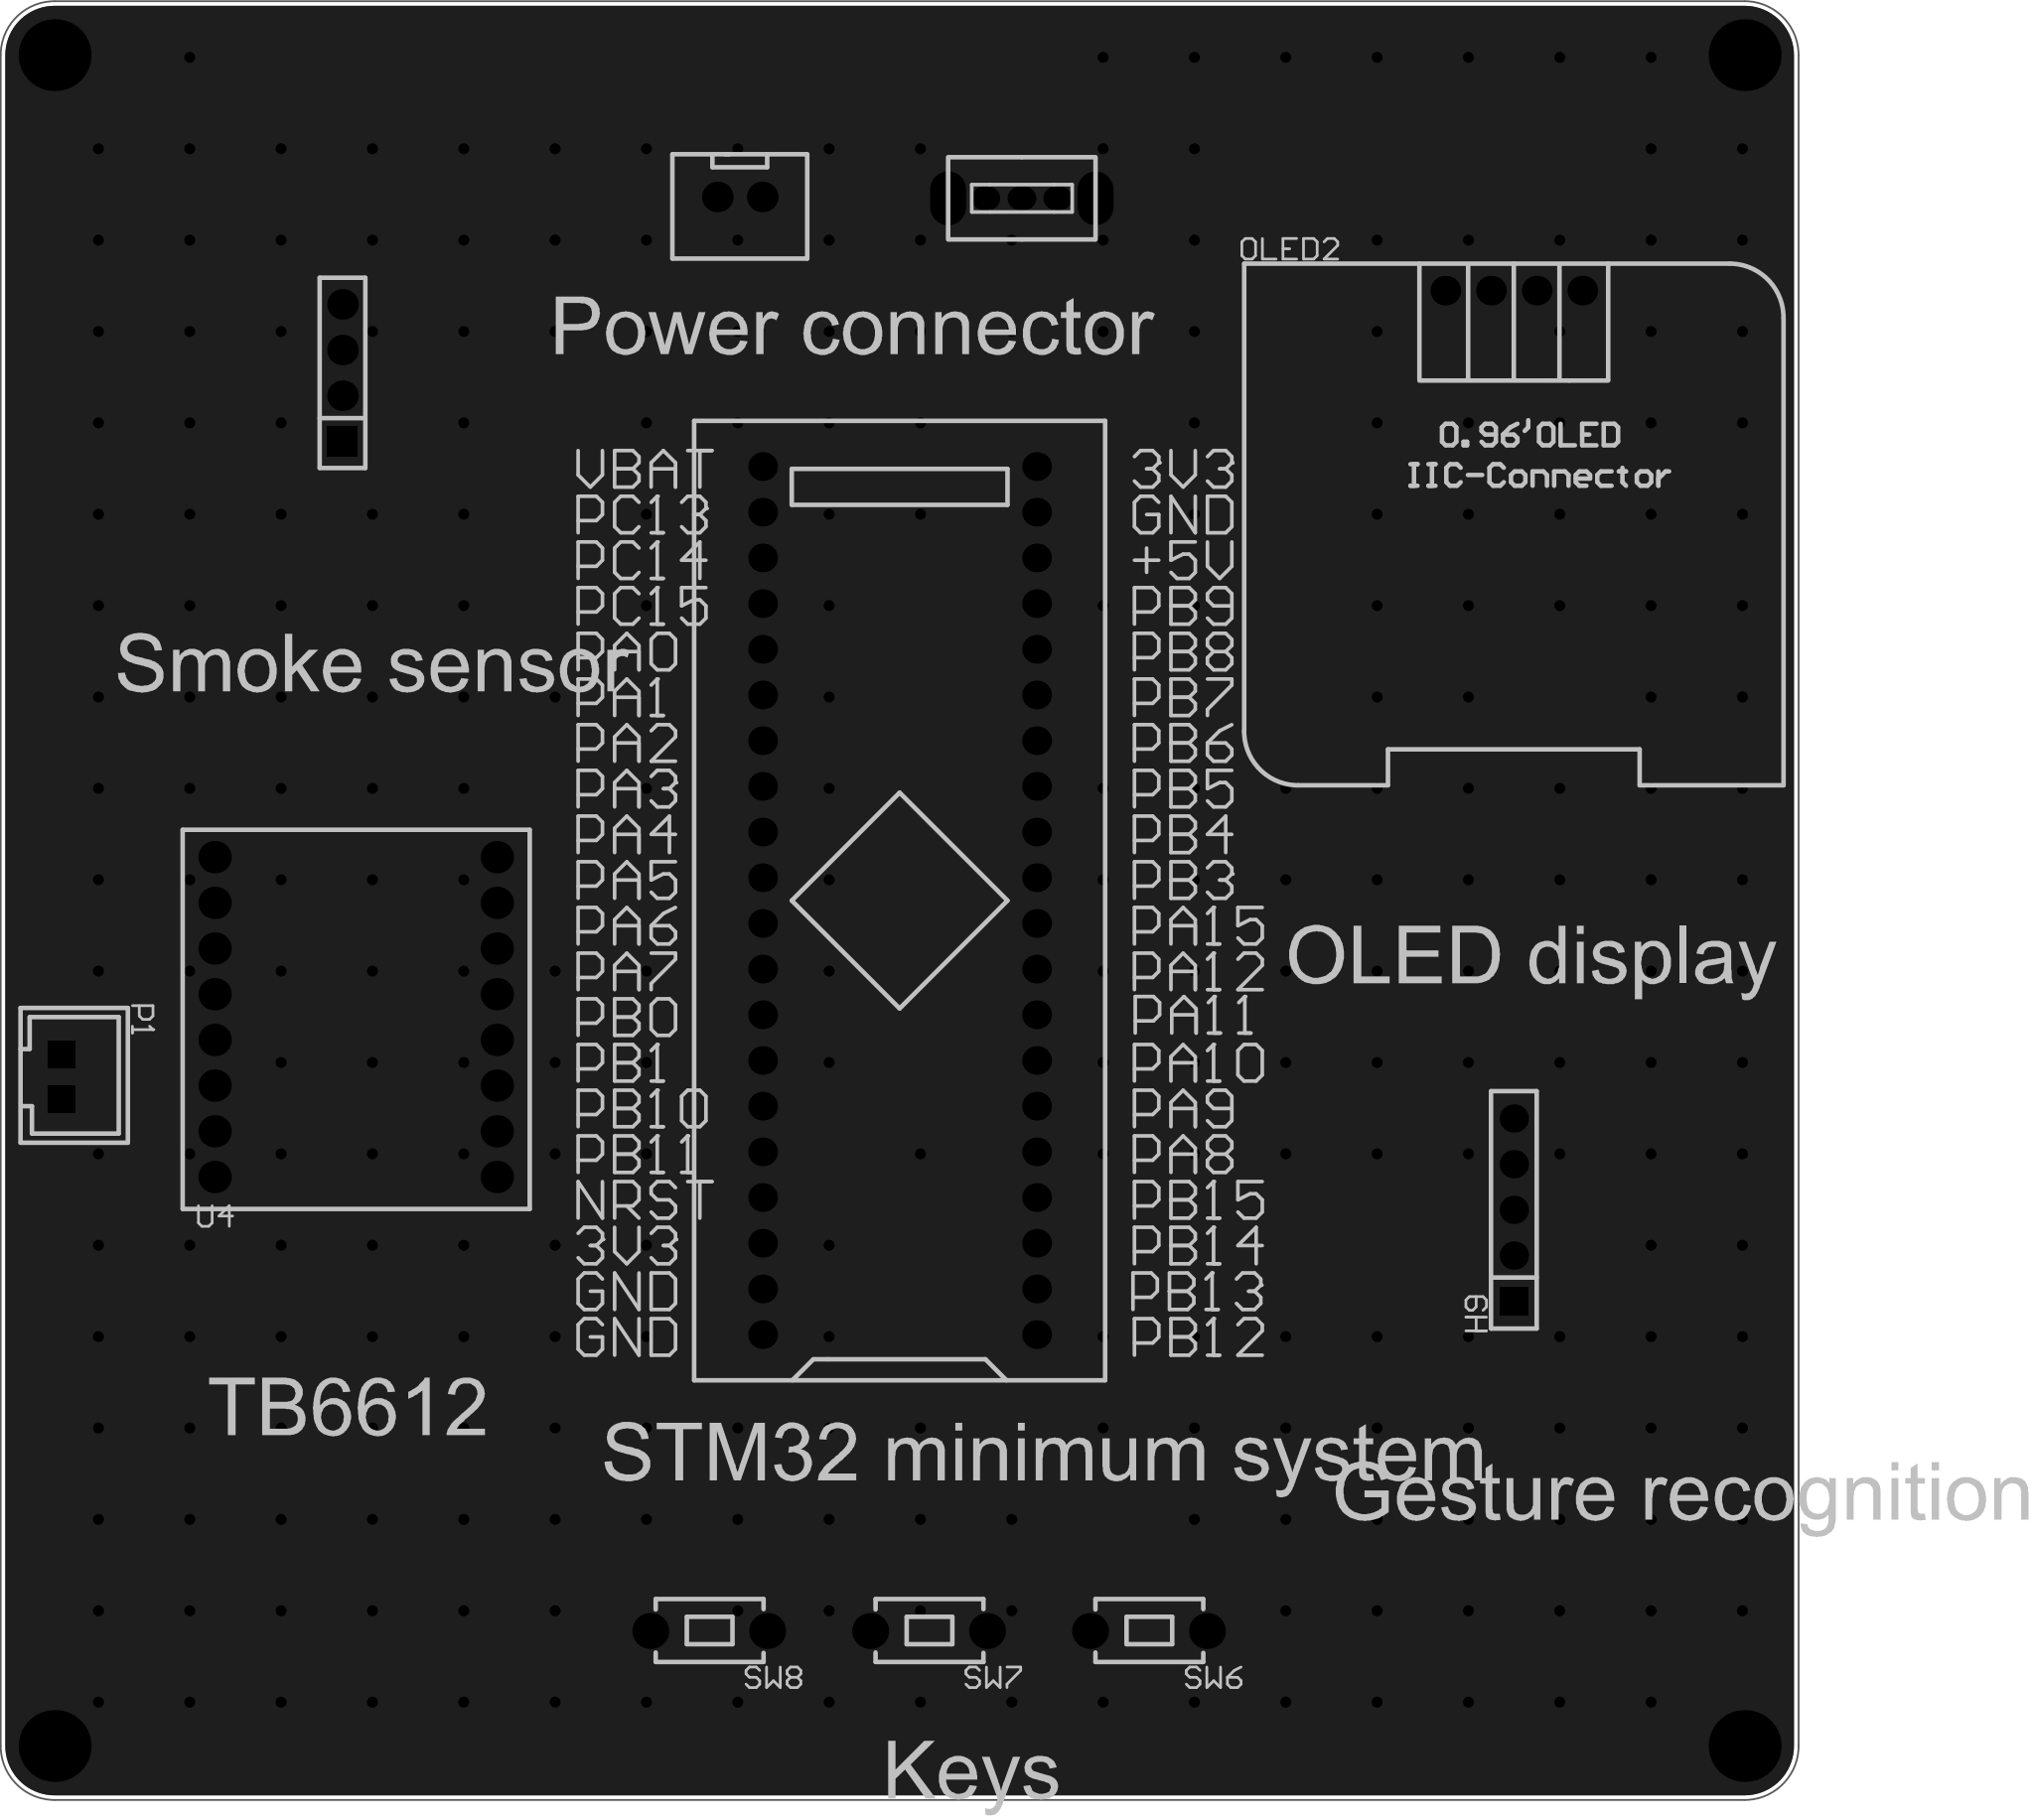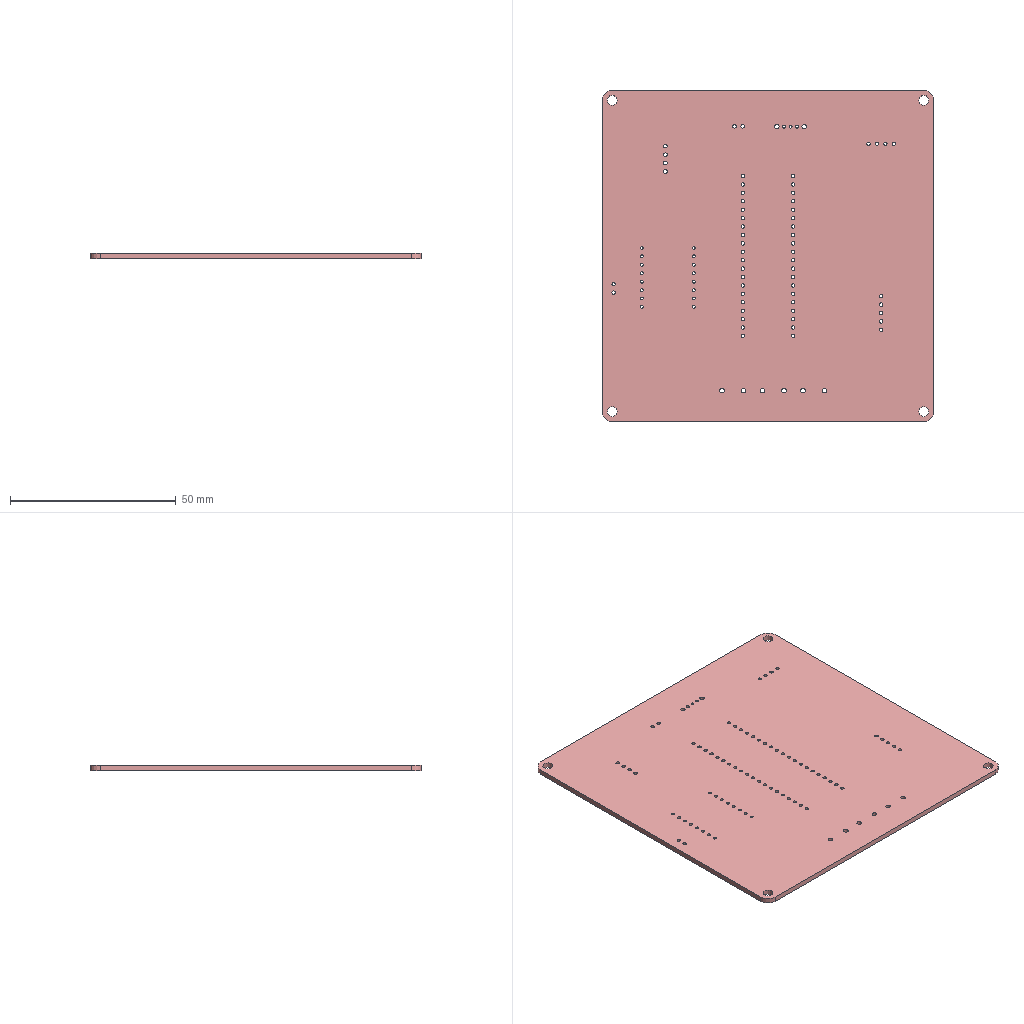Circuit board layout | Altium Designer | box 100 x 100 x 1.6 mm
Layer stack:
# Altium Designer layer stack of  (unit mm; dielectric type: 0 none, 1 core, 2 prepreg, 3 surface material)
index,name,kind,layer,copper_thickness_mm,dielectric_type,dielectric_thickness_mm,dielectric_material,dielectric_constant
0,Top Paste Mask Layer,other,,,,,,
1,Top Silkscreen Layer,other,,,,,,
2,Top Solder Mask Layer,dielectric,,,3,0.01,,3.3
3,Top Layer,copper,Top Layer,0.035,,,,
4,Dielectric1,dielectric,,,3,1.51,FR4,4.5
5,Bottom Layer,copper,Bottom Layer,0.035,,,,
6,Bottom Solder Mask Layer,dielectric,,,3,0.01,,3.3
7,Bottom Silkscreen Layer,other,,,,,,
8,Bottom Paste Mask Layer,other,,,,,,
# drill layer pairs: low layer,high layer
drill_pair,Top Layer,Bottom Layer
Part placement:
Designator,Comment,Layer,Footprint,Center-X(mm),Center-Y(mm),Rotation
U1,STM32F103C8T6-Card,TopLayer,CONN-TH_L53.3-W22.9_STM32F103C8T6-CARD,141.351,130.937,90
CN4,XH2.54*2P_through-hole,TopLayer,CONN-TH_2P-P2.50-XH2.54-2P,132.461,170.053,0
SW5,,TopLayer,拨动开关,148.148,169.978,180
H4,,TopLayer,HDR-TH_4P-P2.54-V-F,110.363,160.274,90
OLED2,,TopLayer,0.96OLED_4P,175.514,164.846,0
H9,,TopLayer,HDR-TH_5P-P2.54-V-F,175.514,113.743,90
SW6,,TopLayer,Key_TH_3.5x6x4.3,155.192,90.33,180
SW7,,TopLayer,Key_TH_3.5x6x4.3,142.963,90.33,180
SW8,,TopLayer,Key_TH_3.5x6x4.3,130.734,90.33,180
U4,,TopLayer,tb6612,111.1,124.46,0
P1,XH2.54 through-hole socket-2P,TopLayer,CONN-TH_XH2.54-2P,94.742,121.158,270
Pad and via stacks:
# Altium Designer via and pad stacks of  (unit mm). Each distinct definition once, with the count of objects using it.
# via: kind,start_layer,end_layer,hole_mm,diameter_mm,mode(0 simple;1 top-mid-bottom;2 full stack),diameter_per_layer,count,example_net
# pad: kind,layer,hole_mm,hole_type(0 round;1 square;2 slot),plating,top_size,top_shape(1 round;2 rect;3 octagon;9 rounded rect),mid_size,bottom_size,mode,footprint,size_per_layer,count,example
pad,Multi-Layer,3,0,plated,4x4,1,4x4,4x4,0,,,4,1
pad,Multi-Layer,1,0,plated,1.6x1.6,1,1.6x1.6,1.6x1.6,0,CONN-TH_L53.3-W22.9_STM32F103C8T6-CARD,,40,U1.1
pad,Multi-Layer,1.05,0,plated,1.7x1.7,1,1.7x1.7,1.7x1.7,0,CONN-TH_2P-P2.50-XH2.54-2P,,2,CN4.2
pad,Multi-Layer,0.8992,0,plated,1.6x1.3,1,1.6x1.3,1.6x1.3,0,\u00B2\u00A6\u00B6\u00AF\u00BF\u00AA\u00B9\u00D8,,3,SW5.1
pad,Multi-Layer,1.3,0,plated,3x1.999,1,3x1.999,3x1.999,0,\u00B2\u00A6\u00B6\u00AF\u00BF\u00AA\u00B9\u00D8,,2,SW5.4
pad,Multi-Layer,1.1,0,plated,1.7x1.7,2,1.7x1.7,1.7x1.7,0,HDR-TH_4P-P2.54-V-F,,1,H4.1
pad,Multi-Layer,1.1,0,plated,1.7x1.7,1,1.7x1.7,1.7x1.7,0,HDR-TH_4P-P2.54-V-F,,3,H4.2
pad,Multi-Layer,1,0,plated,1.65x1.65,1,1.65x1.65,1.65x1.65,0,0.96OLED_4P,,4,OLED2.4
pad,Multi-Layer,1.02,0,plated,1.575x1.575,1,1.575x1.575,1.575x1.575,0,HDR-TH_5P-P2.54-V-F,,4,H9.5
pad,Multi-Layer,1.02,0,plated,1.575x1.575,2,1.575x1.575,1.575x1.575,0,HDR-TH_5P-P2.54-V-F,,1,H9.1
pad,Multi-Layer,1.399,0,plated,1.999x1.999,1,1.999x1.999,1.999x1.999,0,Key_TH_3.5x6x4.3,,6,SW6.A
pad,Multi-Layer,0.9,0,plated,1.8x1.8,1,1.8x1.8,1.8x1.8,0,tb6612,,16,U4.1
pad,Multi-Layer,1,2,plated,1.524x1.524,2,1.524x1.524,1.524x1.524,0,CONN-TH_XH2.54-2P,,2,P1.1
via,Top Layer,Bottom Layer,0.3048,0.61,0,,281,GND
Copper pours:
name,layer,net,type(0 solid;1 hatched;2 none)
Bottom Layer-GND,Bottom Layer,GND,0
Top Layer-GND,Top Layer,GND,0
Design rules, without the lines most boards share:
# Altium Designer design rules of  (exported by Altium Designer, unit mm)
# columns: name | kind | enabled | priority | scope1 | scope2 | descriptor | typed fields (field=value)
Copper_copperRegion_copperThickness1oz | 0 | disabled | 4 | All | All | Clearance Constraint (Gap=5.984mil) (Disabled)(All),(All) | gap=0.152
Copper_copperRegion_copperThickness1oz_1 | 63 | disabled | 4 | All | All | Board Clearance Constraint (Gap=0mil) (Disabled)(All) |
Copper_copperRegion_Copper_copperRegion | 0 | disabled | 5 | All | All | Clearance Constraint (Gap=5.984mil) (Disabled)(All),(All) | gap=0.152
Copper_copperRegion_Copper_copperRegion_1 | 63 | disabled | 5 | All | All | Board Clearance Constraint (Gap=0mil) (Disabled)(All) |
copperThickness1oz | 0 | enabled | 6 | All | All | Clearance Constraint (Gap=5.984mil) (All),(All) | gap=0.152
copperThickness1oz_1 | 63 | enabled | 6 | All | All | Board Clearance Constraint (Gap=0mil) (All) |
copperRegion_copperThickness1oz | 20 | disabled | 1 | All | All | Polygon Connect Rule(Relief Connect )(Conductor Width=10mil) (Relief Angle=90 Angle) (Entries=4) (Air Gap Width=10mil) (Disabled)(All),(All) | connect_style(0=relief,1=direct,2=none)=0 relief_conductor_width=0.254 relief_entries=4
copperRegion_Copper_copperRegion | 20 | disabled | 2 | All | All | Polygon Connect Rule(Relief Connect )(Conductor Width=10mil) (Relief Angle=90 Angle) (Entries=4) (Air Gap Width=10mil) (Disabled)(All),(All) | connect_style(0=relief,1=direct,2=none)=0 relief_conductor_width=0.254 relief_entries=4
copperRegion | 20 | enabled | 3 | All | All | Polygon Connect Rule(Relief Connect )(Conductor Width=10mil) (Relief Angle=90 Angle) (Entries=4) (Air Gap Width=10mil) (All),(All) | connect_style(0=relief,1=direct,2=none)=0 relief_conductor_width=0.254 relief_entries=4